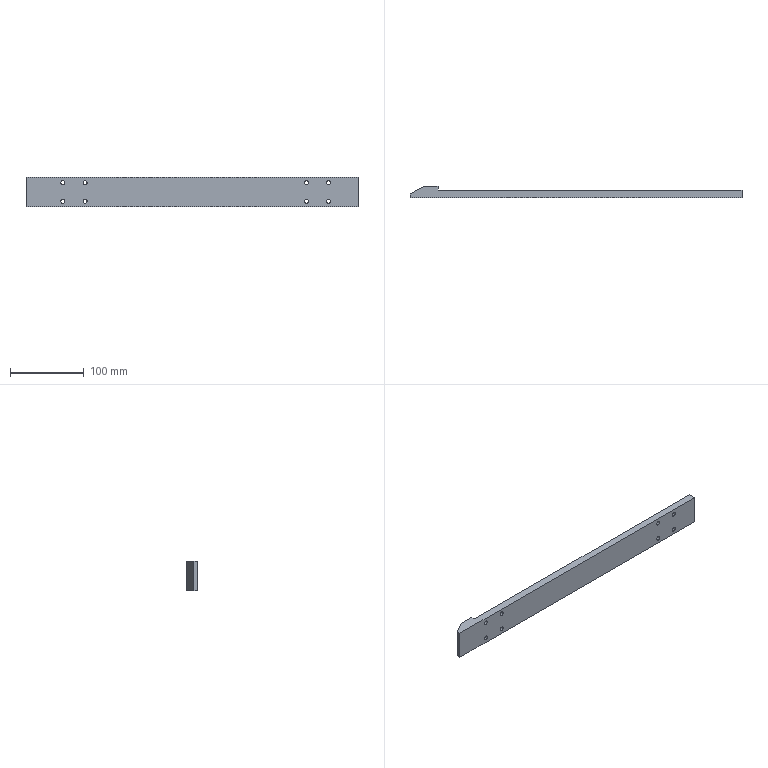Part | SolidWorks | features HoleWzd 2, Extrusion 1 | 1 solid | 57 faces | box 450 x 15 x 40 mm | volume 179202 mm3 | cylinder 36 | plane 17 | cone 4 | commonest cylinder face diameters 5.5 x16 10 x16 4.2 x4